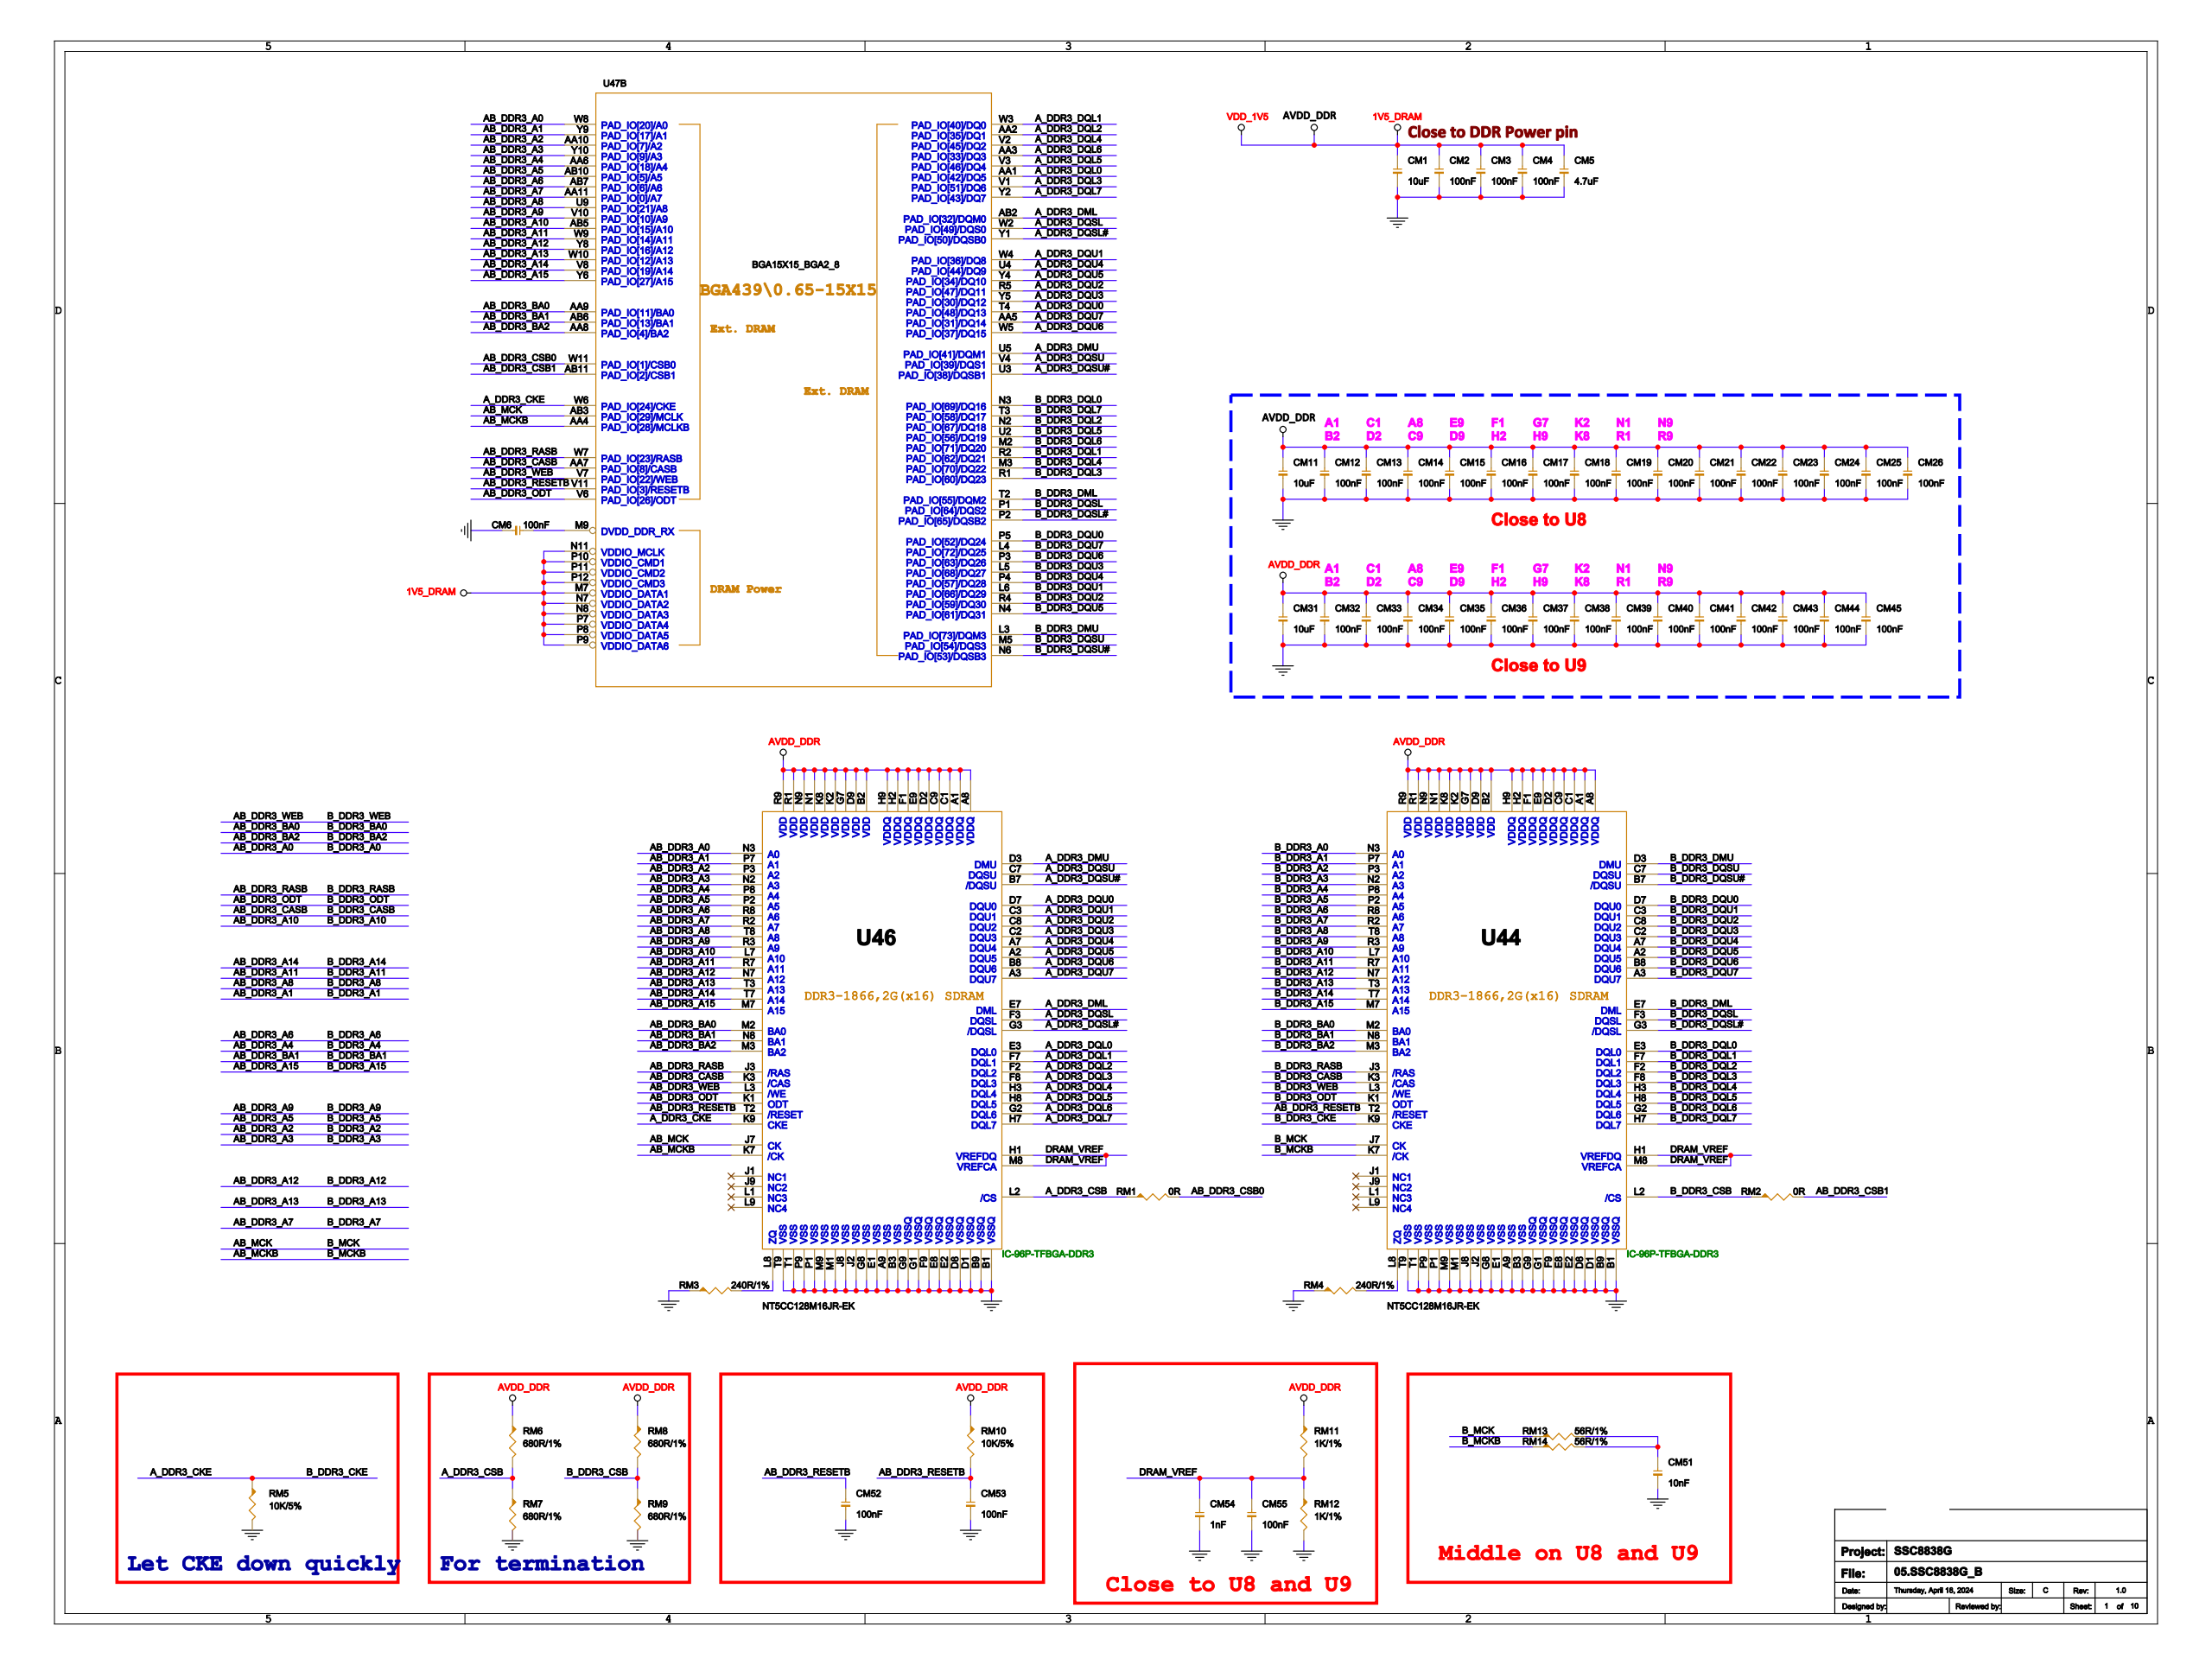Circuit board | Cadence Allegro | 958 parts | 601 nets | one sheet of the schematic
Parts on this sheet (reference | value | footprint):
CM1 | 10uF | C0603
CM2 | 100nF | C0402
CM3 | 100nF | C0402
CM4 | 100nF | C0402
CM5 | 4.7uF | C0402
CM6 | 100nF | C0402
CM11 | 10uF | C0603
CM12 | 100nF | C0402
CM13 | 100nF | C0402
CM14 | 100nF | C0402
CM15 | 100nF | C0402
CM16 | 100nF | C0402
CM17 | 100nF | C0402
CM18 | 100nF | C0402
CM19 | 100nF | C0402
CM20 | 100nF | C0402
CM21 | 100nF | C0402
CM22 | 100nF | C0402
CM23 | 100nF | C0402
CM24 | 100nF | C0402
CM25 | 100nF | C0402
CM26 | 100nF | C0402
CM31 | 10uF | C0603
CM32 | 100nF | C0402
CM33 | 100nF | C0402
CM34 | 100nF | C0402
CM35 | 100nF | C0402
CM36 | 100nF | C0402
CM37 | 100nF | C0402
CM38 | 100nF | C0402
CM39 | 100nF | C0402
CM40 | 100nF | C0402
CM41 | 100nF | C0402
CM42 | 100nF | C0402
CM43 | 100nF | C0402
CM44 | 100nF | C0402
CM45 | 100nF | C0402
CM51 | 10nF | C0402
CM52 | 100nF | C0402
CM53 | 100nF | C0402
CM54 | 1nF | C0402
CM55 | 100nF | C0402
RM1 | 0R | R0402
RM2 | 0R | R0402
RM3 | 240R/1% | R0402
RM4 | 240R/1% | R0402
RM5 | 10K/5% | R0402
RM6 | 680R/1% | R0402
RM7 | 680R/1% | R0402
RM8 | 680R/1% | R0402
RM9 | 680R/1% | R0402
RM10 | 10K/5% | R0402
RM11 | 1K/1% | R0402
RM12 | 1K/1% | R0402
RM13 | 56R/1% | R0402
RM14 | 56R/1% | R0402
U9 | EMMC | BGA153-11_5X13-P0_5-H0_8
U44 | NT5CC128M16JR-EK | IC-96P-TFBGA-DDR3
U46 | NT5CC128M16JR-EK | IC-96P-TFBGA-DDR3
U47 | BGA15X15_BGA2_8 | 8838G
Nets of these parts (net: part-pin ...):
GND: CM1-2 CM2-2 CM3-2 CM4-2 CM5-2 CM6-2 CM11-2 CM12-2 CM13-2 CM14-2 CM15-2 CM16-2 CM17-2 CM18-2 CM19-2 CM20-2 CM21-2 CM22-2 CM23-2 CM24-2 CM25-2 CM26-2 CM31-2 CM32-2 CM33-2 CM34-2 CM35-2 CM36-2 CM37-2 CM38-2 CM39-2 CM40-2 CM41-2 CM42-2 CM43-2 CM44-2 CM45-2 CM51-2 CM52-2 CM53-2 CM54-2 CM55-2 RM3-1 RM4-1 RM5-2 RM7-2 RM9-2 RM12-2 U9-A6 U9-E7 U9-K8 U9-N2 U9-P4 U44-A9 U44-B1 U44-B3 U44-B9 U44-D1 U44-D8 U44-E1 U44-E2 U44-E8 U44-F9 U44-G1 U44-G8 U44-G9 U44-J2 U44-J8 U44-M1 U44-M9 U44-P1 U44-P9 U44-T1 U44-T9 U46-A9 U46-B1 U46-B3 U46-B9 U46-D1 U46-D8 U46-E1 U46-E2 U46-E8 U46-F9 U46-G1 U46-G8 U46-G9 U46-J2 U46-J8 U46-M1 U46-M9 U46-P1 U46-P9 U46-T1 U46-T9 U47-A11 U47-B1 U47-B7 U47-C8 U47-C9 U47-D3 U47-D7 U47-F1 U47-F7 U47-G2 U47-G7 U47-G8 U47-G9 U47-H7 U47-J7 U47-J9 U47-K7 U47-K8 U47-K9 U47-L8 U47-L9 U47-M1 U47-M8 U47-N9 U47-R3 U47-R7 U47-R8 U47-R9 U47-T7 U47-T8 U47-T9 U47-U8
1V5_DRAM: CM1-1 CM2-1 CM3-1 CM4-1 CM5-1 CM11-1 CM12-1 CM13-1 CM14-1 CM15-1 CM16-1 CM17-1 CM18-1 CM19-1 CM20-1 CM21-1 CM22-1 CM23-1 CM24-1 CM25-1 CM26-1 CM31-1 CM32-1 CM33-1 CM34-1 CM35-1 CM36-1 CM37-1 CM38-1 CM39-1 CM40-1 CM41-1 CM42-1 CM43-1 CM44-1 CM45-1 RM6-1 RM8-1 RM10-1 RM11-1 U44-A1 U44-A8 U44-B2 U44-C1 U44-C9 U44-D2 U44-D9 U44-E9 U44-F1 U44-G7 U44-H2 U44-H9 U44-K2 U44-K8 U44-N1 U44-N9 U44-R1 U44-R9 U46-A1 U46-A8 U46-B2 U46-C1 U46-C9 U46-D2 U46-D9 U46-E9 U46-F1 U46-G7 U46-H2 U46-H9 U46-K2 U46-K8 U46-N1 U46-N9 U46-R1 U46-R9 U47-M7 U47-N7 U47-N8 U47-N11 U47-P7 U47-P8 U47-P9 U47-P10 U47-P11 U47-P12
AB_DDR3_RESETB: CM52-1 CM53-1 RM10-2 U44-T2 U46-T2 U47-V11
DRAM_VREF: CM54-1 CM55-1 RM11-2 RM12-1 U44-H1 U44-M8 U46-H1 U46-M8
N20527944: CM6-1 U47-M9
N20528557: CM51-1 RM13-2 RM14-2
A_DDR3_CSB: RM1-1 RM6-2 RM7-1 U46-L2
AB_DDR3_CSB0: RM1-2 U47-W11
B_DDR3_CSB: RM2-1 RM8-2 RM9-1 U44-L2
AB_DDR3_CSB1: RM2-2 U47-AB11
A_DDR3_CKE: RM5-1 U44-K9 U46-K9 U47-W6
AB_MCK: RM13-1 U44-J7 U46-J7 U47-AB3
AB_MCKB: RM14-1 U44-K7 U46-K7 U47-AA4
N20527014: RM3-2 U46-L8
N20527565: RM4-2 U44-L8
B_DDR3_DQU5: U44-A2 U47-N4
B_DDR3_DQU7: U44-A3 U47-L4
B_DDR3_DQU4: U44-A7 U47-P4
B_DDR3_DQSU#: U44-B7 U47-N6
B_DDR3_DQU6: U44-B8 U47-P3
B_DDR3_DQU3: U44-C2 U47-L5
B_DDR3_DQU1: U44-C3 U47-L6
B_DDR3_DQSU: U44-C7 U47-M5
B_DDR3_DQU2: U44-C8 U47-R4
B_DDR3_DMU: U44-D3 U47-L3
B_DDR3_DQU0: U44-D7 U47-P5
B_DDR3_DQL0: U44-E3 U47-N3
B_DDR3_DML: U44-E7 U47-T2
B_DDR3_DQL2: U44-F2 U47-N2
B_DDR3_DQSL: U44-F3 U47-P1
B_DDR3_DQL1: U44-F7 U47-R2
B_DDR3_DQL3: U44-F8 U47-R1
B_DDR3_DQL6: U44-G2 U47-M2
B_DDR3_DQSL#: U44-G3 U47-P2
B_DDR3_DQL4: U44-H3 U47-M3
B_DDR3_DQL7: U44-H7 U47-T3
B_DDR3_DQL5: U44-H8 U47-U2
AB_DDR3_RASB: U44-J3 U46-J3 U47-W7
AB_DDR3_ODT: U44-K1 U46-K1 U47-V6
AB_DDR3_CASB: U44-K3 U46-K3 U47-AA7
AB_DDR3_WEB: U44-L3 U46-L3 U47-V7
AB_DDR3_A10: U44-L7 U46-L7 U47-AB5
AB_DDR3_BA0: U44-M2 U46-M2 U47-AA9
AB_DDR3_BA2: U44-M3 U46-M3 U47-AA8
AB_DDR3_A15: U44-M7 U46-M7 U47-Y6
AB_DDR3_A3: U44-N2 U46-N2 U47-Y10
AB_DDR3_A0: U44-N3 U46-N3 U47-W8
AB_DDR3_A12: U44-N7 U46-N7 U47-Y8
AB_DDR3_BA1: U44-N8 U46-N8 U47-AB6
AB_DDR3_A5: U44-P2 U46-P2 U47-AB10
AB_DDR3_A2: U44-P3 U46-P3 U47-AA10
AB_DDR3_A1: U44-P7 U46-P7 U47-Y9
AB_DDR3_A4: U44-P8 U46-P8 U47-AA6
AB_DDR3_A7: U44-R2 U46-R2 U47-AA11
AB_DDR3_A9: U44-R3 U46-R3 U47-V10
AB_DDR3_A11: U44-R7 U46-R7 U47-W9
AB_DDR3_A6: U44-R8 U46-R8 U47-AB7
AB_DDR3_A13: U44-T3 U46-T3 U47-W10
AB_DDR3_A14: U44-T7 U46-T7 U47-V8
AB_DDR3_A8: U44-T8 U46-T8 U47-U9
A_DDR3_DQU5: U46-A2 U47-Y4
A_DDR3_DQU7: U46-A3 U47-AA5
A_DDR3_DQU4: U46-A7 U47-U4
A_DDR3_DQSU#: U46-B7 U47-U3
A_DDR3_DQU6: U46-B8 U47-W5
A_DDR3_DQU3: U46-C2 U47-Y5
A_DDR3_DQU1: U46-C3 U47-W4
A_DDR3_DQSU: U46-C7 U47-V4
A_DDR3_DQU2: U46-C8 U47-R5
A_DDR3_DMU: U46-D3 U47-U5
A_DDR3_DQU0: U46-D7 U47-T4
A_DDR3_DQL0: U46-E3 U47-AA1
A_DDR3_DML: U46-E7 U47-AB2
A_DDR3_DQL2: U46-F2 U47-AA2
A_DDR3_DQSL: U46-F3 U47-W2
A_DDR3_DQL1: U46-F7 U47-W3
A_DDR3_DQL3: U46-F8 U47-V1
A_DDR3_DQL6: U46-G2 U47-AA3
A_DDR3_DQSL#: U46-G3 U47-Y1
A_DDR3_DQL4: U46-H3 U47-V2
A_DDR3_DQL7: U46-H7 U47-Y2
A_DDR3_DQL5: U46-H8 U47-V3